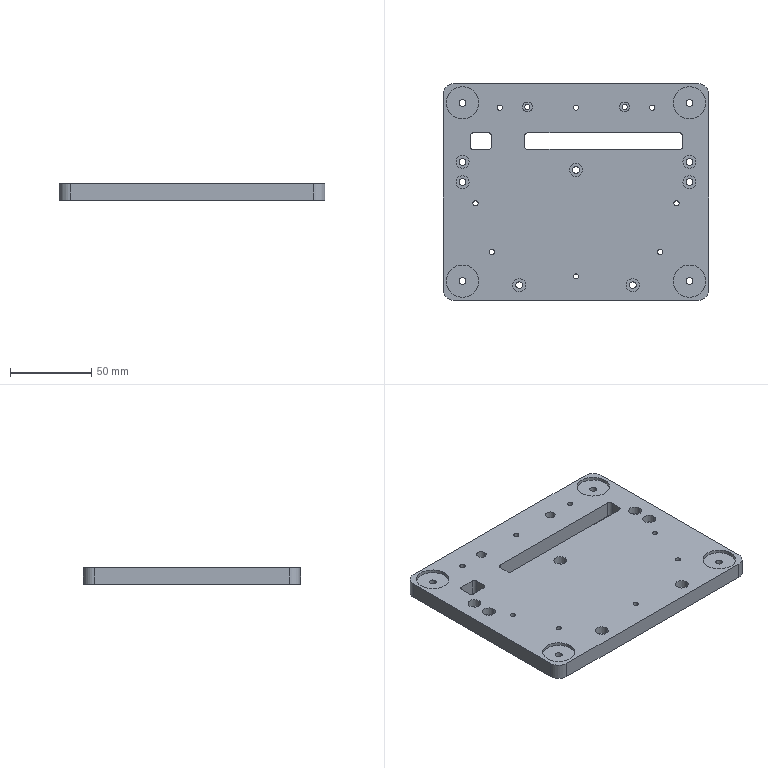Part | SolidWorks | features BaseBody 1 | 1 solid | 131 faces | box 164 x 134 x 10 mm | volume 201088 mm3 | cylinder 88 | plane 35 | spline 8 | commonest cylinder face diameters 4.2 x22 8 x14 3.2 x12 6 x12 3.3 x8 20 x8